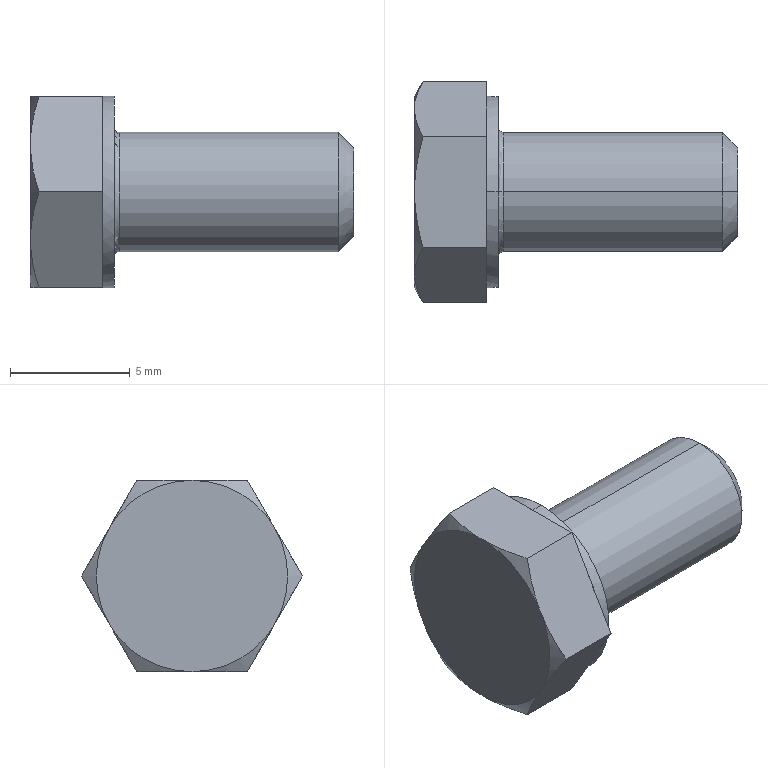Part | SolidWorks | features RevCut 4, Chamfer 1, Extrusion 1, Fillet 1, LPattern 1, Revolution 1 | 1 solid | 29 faces | box 13.5 x 9.238 x 8 mm | volume 384.396 mm3 | plane 15 | cone 8 | cylinder 4 | torus 2 | commonest cylinder face diameters 5 x2 8 x2
STEP:
#1=CARTESIAN_POINT('',(3.7,0.,2.5));
#2=VERTEX_POINT('',#1);
#3=CARTESIAN_POINT('',(3.7,0.,-2.5));
#4=VERTEX_POINT('',#3);
#5=CARTESIAN_POINT('',(3.7,0.,0.));
#6=DIRECTION('',(1.,0.,0.));
#7=DIRECTION('',(0.,0.,-1.));
#8=AXIS2_PLACEMENT_3D('',#5,#6,#7);
#9=CIRCLE('',#8,2.5);
#10=EDGE_CURVE('',#2,#4,#9,.T.);
#11=ORIENTED_EDGE('',*,*,#10,.F.);
#12=CARTESIAN_POINT('',(3.5,0.,2.7));
#13=VERTEX_POINT('',#12);
#14=CARTESIAN_POINT('',(3.7,0.,2.7));
#15=DIRECTION('',(0.,1.,0.));
#16=DIRECTION('',(0.,0.,1.));
#17=AXIS2_PLACEMENT_3D('',#14,#15,#16);
#18=CIRCLE('',#17,0.2);
#19=EDGE_CURVE('',#2,#13,#18,.T.);
#20=ORIENTED_EDGE('',*,*,#19,.T.);
#21=CARTESIAN_POINT('',(3.5,0.,-2.7));
#22=VERTEX_POINT('',#21);
#23=CARTESIAN_POINT('',(3.5,0.,0.));
#24=DIRECTION('',(-1.,0.,0.));
#25=DIRECTION('',(0.,0.,-1.));
#26=AXIS2_PLACEMENT_3D('',#23,#24,#25);
#27=CIRCLE('',#26,2.7);
#28=EDGE_CURVE('',#22,#13,#27,.T.);
#29=ORIENTED_EDGE('',*,*,#28,.F.);
#30=CARTESIAN_POINT('',(3.7,0.,-2.7));
#31=DIRECTION('',(0.,-1.,0.));
#32=DIRECTION('',(0.,0.,-1.));
#33=AXIS2_PLACEMENT_3D('',#30,#31,#32);
#34=CIRCLE('',#33,0.2);
#35=EDGE_CURVE('',#4,#22,#34,.T.);
#36=ORIENTED_EDGE('',*,*,#35,.F.);
#37=EDGE_LOOP('',(#11,#20,#29,#36));
#38=FACE_OUTER_BOUND('',#37,.T.);
#39=CARTESIAN_POINT('',(3.7,0.,0.));
#40=DIRECTION('',(1.,0.,0.));
#41=DIRECTION('',(0.,0.,-1.));
#42=AXIS2_PLACEMENT_3D('',#39,#40,#41);
#43=TOROIDAL_SURFACE('',#42,2.7,0.2);
#44=ADVANCED_FACE('',(#38),#43,.F.);
#45=CARTESIAN_POINT('',(13.5,0.,-1.86));
#46=VERTEX_POINT('',#45);
#47=CARTESIAN_POINT('',(13.5,0.,1.86));
#48=VERTEX_POINT('',#47);
#49=CARTESIAN_POINT('',(13.5,0.,0.));
#50=DIRECTION('',(1.,0.,0.));
#51=DIRECTION('',(0.,0.,1.));
#52=AXIS2_PLACEMENT_3D('',#49,#50,#51);
#53=CIRCLE('',#52,1.86);
#54=EDGE_CURVE('',#46,#48,#53,.T.);
#55=ORIENTED_EDGE('',*,*,#54,.F.);
#56=CARTESIAN_POINT('',(12.86,0.,-2.5));
#57=VERTEX_POINT('',#56);
#58=CARTESIAN_POINT('',(12.86,0.,-2.5));
#59=DIRECTION('',(-0.7071,0.,-0.7071));
#60=VECTOR('',#59,1000.);
#61=LINE('',#58,#60);
#62=EDGE_CURVE('',#46,#57,#61,.T.);
#63=ORIENTED_EDGE('',*,*,#62,.T.);
#64=CARTESIAN_POINT('',(12.86,0.,2.5));
#65=VERTEX_POINT('',#64);
#66=CARTESIAN_POINT('',(12.86,0.,0.));
#67=DIRECTION('',(-1.,0.,0.));
#68=DIRECTION('',(0.,0.,1.));
#69=AXIS2_PLACEMENT_3D('',#66,#67,#68);
#70=CIRCLE('',#69,2.5);
#71=EDGE_CURVE('',#65,#57,#70,.T.);
#72=ORIENTED_EDGE('',*,*,#71,.F.);
#73=CARTESIAN_POINT('',(12.86,0.,2.5));
#74=DIRECTION('',(-0.7071,0.,0.7071));
#75=VECTOR('',#74,1000.);
#76=LINE('',#73,#75);
#77=EDGE_CURVE('',#48,#65,#76,.T.);
#78=ORIENTED_EDGE('',*,*,#77,.F.);
#79=EDGE_LOOP('',(#55,#63,#72,#78));
#80=FACE_OUTER_BOUND('',#79,.T.);
#81=CARTESIAN_POINT('',(12.86,0.,0.));
#82=DIRECTION('',(-1.,0.,0.));
#83=DIRECTION('',(0.,0.,1.));
#84=AXIS2_PLACEMENT_3D('',#81,#82,#83);
#85=CONICAL_SURFACE('',#84,2.5,0.7854);
#86=ADVANCED_FACE('',(#80),#85,.T.);
#87=ORIENTED_EDGE('',*,*,#71,.T.);
#88=CARTESIAN_POINT('',(0.,0.,-2.5));
#89=DIRECTION('',(-1.,0.,0.));
#90=VECTOR('',#89,1000.);
#91=LINE('',#88,#90);
#92=EDGE_CURVE('',#57,#4,#91,.T.);
#93=ORIENTED_EDGE('',*,*,#92,.T.);
#94=CARTESIAN_POINT('',(3.7,0.,0.));
#95=DIRECTION('',(1.,0.,0.));
#96=DIRECTION('',(0.,0.,-1.));
#97=AXIS2_PLACEMENT_3D('',#94,#95,#96);
#98=CIRCLE('',#97,2.5);
#99=EDGE_CURVE('',#4,#2,#98,.T.);
#100=ORIENTED_EDGE('',*,*,#99,.T.);
#101=CARTESIAN_POINT('',(0.,0.,2.5));
#102=DIRECTION('',(-1.,0.,0.));
#103=VECTOR('',#102,1000.);
#104=LINE('',#101,#103);
#105=EDGE_CURVE('',#65,#2,#104,.T.);
#106=ORIENTED_EDGE('',*,*,#105,.F.);
#107=EDGE_LOOP('',(#87,#93,#100,#106));
#108=FACE_OUTER_BOUND('',#107,.T.);
#109=CARTESIAN_POINT('',(0.,0.,0.));
#110=DIRECTION('',(-1.,0.,0.));
#111=DIRECTION('',(0.,0.,1.));
#112=AXIS2_PLACEMENT_3D('',#109,#110,#111);
#113=CYLINDRICAL_SURFACE('',#112,2.5);
#114=ADVANCED_FACE('',(#108),#113,.T.);
#115=CARTESIAN_POINT('',(3.5,0.,-4.));
#116=VERTEX_POINT('',#115);
#117=CARTESIAN_POINT('',(3.5,0.,4.));
#118=VERTEX_POINT('',#117);
#119=CARTESIAN_POINT('',(3.5,0.,0.));
#120=DIRECTION('',(1.,0.,0.));
#121=DIRECTION('',(0.,0.,-1.));
#122=AXIS2_PLACEMENT_3D('',#119,#120,#121);
#123=CIRCLE('',#122,4.);
#124=EDGE_CURVE('',#116,#118,#123,.T.);
#125=ORIENTED_EDGE('',*,*,#124,.F.);
#126=CARTESIAN_POINT('',(3.,0.,-4.));
#127=VERTEX_POINT('',#126);
#128=CARTESIAN_POINT('',(0.,0.,-4.));
#129=DIRECTION('',(-1.,0.,0.));
#130=VECTOR('',#129,1000.);
#131=LINE('',#128,#130);
#132=EDGE_CURVE('',#116,#127,#131,.T.);
#133=ORIENTED_EDGE('',*,*,#132,.T.);
#134=CARTESIAN_POINT('',(3.,3.464,-2.));
#135=VERTEX_POINT('',#134);
#136=CARTESIAN_POINT('',(3.,0.,0.));
#137=DIRECTION('',(-1.,0.,0.));
#138=DIRECTION('',(0.,0.,1.));
#139=AXIS2_PLACEMENT_3D('',#136,#137,#138);
#140=CIRCLE('',#139,4.);
#141=EDGE_CURVE('',#135,#127,#140,.T.);
#142=ORIENTED_EDGE('',*,*,#141,.F.);
#143=CARTESIAN_POINT('',(3.,3.464,2.));
#144=VERTEX_POINT('',#143);
#145=CARTESIAN_POINT('',(3.,0.,0.));
#146=DIRECTION('',(-1.,0.,0.));
#147=DIRECTION('',(0.,0.,1.));
#148=AXIS2_PLACEMENT_3D('',#145,#146,#147);
#149=CIRCLE('',#148,4.);
#150=EDGE_CURVE('',#144,#135,#149,.T.);
#151=ORIENTED_EDGE('',*,*,#150,.F.);
#152=CARTESIAN_POINT('',(3.,0.,4.));
#153=VERTEX_POINT('',#152);
#154=CARTESIAN_POINT('',(3.,0.,0.));
#155=DIRECTION('',(-1.,0.,0.));
#156=DIRECTION('',(0.,0.,1.));
#157=AXIS2_PLACEMENT_3D('',#154,#155,#156);
#158=CIRCLE('',#157,4.);
#159=EDGE_CURVE('',#153,#144,#158,.T.);
#160=ORIENTED_EDGE('',*,*,#159,.F.);
#161=CARTESIAN_POINT('',(0.,0.,4.));
#162=DIRECTION('',(-1.,0.,0.));
#163=VECTOR('',#162,1000.);
#164=LINE('',#161,#163);
#165=EDGE_CURVE('',#118,#153,#164,.T.);
#166=ORIENTED_EDGE('',*,*,#165,.F.);
#167=EDGE_LOOP('',(#125,#133,#142,#151,#160,#166));
#168=FACE_OUTER_BOUND('',#167,.T.);
#169=CARTESIAN_POINT('',(0.,0.,0.));
#170=DIRECTION('',(-1.,0.,0.));
#171=DIRECTION('',(0.,0.,1.));
#172=AXIS2_PLACEMENT_3D('',#169,#170,#171);
#173=CYLINDRICAL_SURFACE('',#172,4.);
#174=ADVANCED_FACE('',(#168),#173,.T.);
#175=CARTESIAN_POINT('',(3.,2.309,-4.));
#176=VERTEX_POINT('',#175);
#177=CARTESIAN_POINT('',(3.,2.309,-4.));
#178=DIRECTION('',(0.,0.5,0.866));
#179=VECTOR('',#178,1000.);
#180=LINE('',#177,#179);
#181=EDGE_CURVE('',#176,#135,#180,.T.);
#182=ORIENTED_EDGE('',*,*,#181,.F.);
#183=CARTESIAN_POINT('',(0.3573,2.309,-4.));
#184=VERTEX_POINT('',#183);
#185=CARTESIAN_POINT('',(3.5,2.309,-4.));
#186=DIRECTION('',(-1.,0.,0.));
#187=VECTOR('',#186,1000.);
#188=LINE('',#185,#187);
#189=EDGE_CURVE('',#176,#184,#188,.T.);
#190=ORIENTED_EDGE('',*,*,#189,.T.);
#191=CARTESIAN_POINT('',(0.,3.464,-2.));
#192=VERTEX_POINT('',#191);
#193=CARTESIAN_POINT('',(0.,3.464,-2.));
#194=CARTESIAN_POINT('',(0.,3.268,-2.339));
#195=CARTESIAN_POINT('',(0.03421,3.072,-2.678));
#196=CARTESIAN_POINT('',(0.1587,2.688,-3.345));
#197=CARTESIAN_POINT('',(0.2485,2.498,-3.674));
#198=CARTESIAN_POINT('',(0.3573,2.309,-4.));
#199=B_SPLINE_CURVE_WITH_KNOTS('',3,(#193,#194,#195,#196,#197,#198),.UNSPECIFIED.,.F.,.F.,(4,2,4),(0.002337,0.003501,0.004665),.UNSPECIFIED.);
#200=EDGE_CURVE('',#192,#184,#199,.T.);
#201=ORIENTED_EDGE('',*,*,#200,.F.);
#202=CARTESIAN_POINT('',(0.3573,4.619,0.));
#203=VERTEX_POINT('',#202);
#204=CARTESIAN_POINT('',(0.3573,4.619,0.));
#205=CARTESIAN_POINT('',(0.1392,4.241,-0.6543));
#206=CARTESIAN_POINT('',(0.,3.858,-1.319));
#207=CARTESIAN_POINT('',(0.,3.464,-2.));
#208=B_SPLINE_CURVE_WITH_KNOTS('',3,(#204,#205,#206,#207),.UNSPECIFIED.,.F.,.F.,(4,4),(0.000000238,0.002337),.UNSPECIFIED.);
#209=EDGE_CURVE('',#203,#192,#208,.T.);
#210=ORIENTED_EDGE('',*,*,#209,.F.);
#211=CARTESIAN_POINT('',(3.,4.619,0.));
#212=VERTEX_POINT('',#211);
#213=CARTESIAN_POINT('',(3.5,4.619,0.));
#214=DIRECTION('',(-1.,0.,0.));
#215=VECTOR('',#214,1000.);
#216=LINE('',#213,#215);
#217=EDGE_CURVE('',#212,#203,#216,.T.);
#218=ORIENTED_EDGE('',*,*,#217,.F.);
#219=CARTESIAN_POINT('',(3.,2.309,-4.));
#220=DIRECTION('',(0.,0.5,0.866));
#221=VECTOR('',#220,1000.);
#222=LINE('',#219,#221);
#223=EDGE_CURVE('',#135,#212,#222,.T.);
#224=ORIENTED_EDGE('',*,*,#223,.F.);
#225=EDGE_LOOP('',(#182,#190,#201,#210,#218,#224));
#226=FACE_OUTER_BOUND('',#225,.T.);
#227=CARTESIAN_POINT('',(3.5,2.309,-4.));
#228=DIRECTION('',(0.,-0.866,0.5));
#229=DIRECTION('',(0.,-0.5,-0.866));
#230=AXIS2_PLACEMENT_3D('',#227,#228,#229);
#231=PLANE('',#230);
#232=ADVANCED_FACE('',(#226),#231,.F.);
#233=CARTESIAN_POINT('',(3.,4.619,0.));
#234=DIRECTION('',(0.,-0.5,0.866));
#235=VECTOR('',#234,1000.);
#236=LINE('',#233,#235);
#237=EDGE_CURVE('',#212,#144,#236,.T.);
#238=ORIENTED_EDGE('',*,*,#237,.F.);
#239=ORIENTED_EDGE('',*,*,#217,.T.);
#240=CARTESIAN_POINT('',(0.,3.464,2.));
#241=VERTEX_POINT('',#240);
#242=CARTESIAN_POINT('',(0.,3.464,2.));
#243=CARTESIAN_POINT('',(0.,3.66,1.661));
#244=CARTESIAN_POINT('',(0.03421,3.856,1.322));
#245=CARTESIAN_POINT('',(0.1587,4.24,0.6554));
#246=CARTESIAN_POINT('',(0.2485,4.43,0.3264));
#247=CARTESIAN_POINT('',(0.3573,4.619,0.));
#248=B_SPLINE_CURVE_WITH_KNOTS('',3,(#242,#243,#244,#245,#246,#247),.UNSPECIFIED.,.F.,.F.,(4,2,4),(0.002337,0.003501,0.004665),.UNSPECIFIED.);
#249=EDGE_CURVE('',#241,#203,#248,.T.);
#250=ORIENTED_EDGE('',*,*,#249,.F.);
#251=CARTESIAN_POINT('',(0.3573,2.309,4.));
#252=VERTEX_POINT('',#251);
#253=CARTESIAN_POINT('',(0.3573,2.309,4.));
#254=CARTESIAN_POINT('',(0.1392,2.687,3.346));
#255=CARTESIAN_POINT('',(0.,3.071,2.681));
#256=CARTESIAN_POINT('',(0.,3.464,2.));
#257=B_SPLINE_CURVE_WITH_KNOTS('',3,(#253,#254,#255,#256),.UNSPECIFIED.,.F.,.F.,(4,4),(0.000000238,0.002337),.UNSPECIFIED.);
#258=EDGE_CURVE('',#252,#241,#257,.T.);
#259=ORIENTED_EDGE('',*,*,#258,.F.);
#260=CARTESIAN_POINT('',(3.,2.309,4.));
#261=VERTEX_POINT('',#260);
#262=CARTESIAN_POINT('',(3.5,2.309,4.));
#263=DIRECTION('',(-1.,0.,0.));
#264=VECTOR('',#263,1000.);
#265=LINE('',#262,#264);
#266=EDGE_CURVE('',#261,#252,#265,.T.);
#267=ORIENTED_EDGE('',*,*,#266,.F.);
#268=CARTESIAN_POINT('',(3.,4.619,0.));
#269=DIRECTION('',(0.,-0.5,0.866));
#270=VECTOR('',#269,1000.);
#271=LINE('',#268,#270);
#272=EDGE_CURVE('',#144,#261,#271,.T.);
#273=ORIENTED_EDGE('',*,*,#272,.F.);
#274=EDGE_LOOP('',(#238,#239,#250,#259,#267,#273));
#275=FACE_OUTER_BOUND('',#274,.T.);
#276=CARTESIAN_POINT('',(3.5,4.619,0.));
#277=DIRECTION('',(0.,-0.866,-0.5));
#278=DIRECTION('',(0.,0.5,-0.866));
#279=AXIS2_PLACEMENT_3D('',#276,#277,#278);
#280=PLANE('',#279);
#281=ADVANCED_FACE('',(#275),#280,.F.);
#282=CARTESIAN_POINT('',(3.,2.309,4.));
#283=DIRECTION('',(0.,-1.,0.));
#284=VECTOR('',#283,1000.);
#285=LINE('',#282,#284);
#286=EDGE_CURVE('',#261,#153,#285,.T.);
#287=ORIENTED_EDGE('',*,*,#286,.F.);
#288=ORIENTED_EDGE('',*,*,#266,.T.);
#289=CARTESIAN_POINT('',(0.,0.,4.));
#290=VERTEX_POINT('',#289);
#291=CARTESIAN_POINT('',(0.,0.,4.));
#292=CARTESIAN_POINT('',(0.,0.3912,4.));
#293=CARTESIAN_POINT('',(0.03459,0.7871,4.));
#294=CARTESIAN_POINT('',(0.1597,1.558,4.));
#295=CARTESIAN_POINT('',(0.2494,1.936,4.));
#296=CARTESIAN_POINT('',(0.3573,2.309,4.));
#297=B_SPLINE_CURVE_WITH_KNOTS('',3,(#291,#292,#293,#294,#295,#296),.UNSPECIFIED.,.F.,.F.,(4,2,4),(0.006655,0.007825,0.008995),.UNSPECIFIED.);
#298=EDGE_CURVE('',#290,#252,#297,.T.);
#299=ORIENTED_EDGE('',*,*,#298,.F.);
#300=CARTESIAN_POINT('',(0.3573,-2.309,4.));
#301=VERTEX_POINT('',#300);
#302=CARTESIAN_POINT('',(0.3573,-2.309,4.));
#303=CARTESIAN_POINT('',(0.2487,-1.933,4.));
#304=CARTESIAN_POINT('',(0.1579,-1.549,4.));
#305=CARTESIAN_POINT('',(0.03364,-0.7786,4.));
#306=CARTESIAN_POINT('',(0.,-0.3909,4.));
#307=CARTESIAN_POINT('',(0.,0.,4.));
#308=B_SPLINE_CURVE_WITH_KNOTS('',3,(#302,#303,#304,#305,#306,#307),.UNSPECIFIED.,.F.,.F.,(4,2,4),(0.004317,0.005486,0.006655),.UNSPECIFIED.);
#309=EDGE_CURVE('',#301,#290,#308,.T.);
#310=ORIENTED_EDGE('',*,*,#309,.F.);
#311=CARTESIAN_POINT('',(3.,-2.309,4.));
#312=VERTEX_POINT('',#311);
#313=CARTESIAN_POINT('',(3.5,-2.309,4.));
#314=DIRECTION('',(-1.,0.,0.));
#315=VECTOR('',#314,1000.);
#316=LINE('',#313,#315);
#317=EDGE_CURVE('',#312,#301,#316,.T.);
#318=ORIENTED_EDGE('',*,*,#317,.F.);
#319=CARTESIAN_POINT('',(3.,2.309,4.));
#320=DIRECTION('',(0.,-1.,0.));
#321=VECTOR('',#320,1000.);
#322=LINE('',#319,#321);
#323=EDGE_CURVE('',#153,#312,#322,.T.);
#324=ORIENTED_EDGE('',*,*,#323,.F.);
#325=EDGE_LOOP('',(#287,#288,#299,#310,#318,#324));
#326=FACE_OUTER_BOUND('',#325,.T.);
#327=CARTESIAN_POINT('',(3.5,2.309,4.));
#328=DIRECTION('',(0.,0.,-1.));
#329=DIRECTION('',(0.,1.,0.));
#330=AXIS2_PLACEMENT_3D('',#327,#328,#329);
#331=PLANE('',#330);
#332=ADVANCED_FACE('',(#326),#331,.F.);
#333=CARTESIAN_POINT('',(3.,-3.464,2.));
#334=VERTEX_POINT('',#333);
#335=CARTESIAN_POINT('',(3.,-4.619,0.));
#336=DIRECTION('',(0.,-0.5,-0.866));
#337=VECTOR('',#336,1000.);
#338=LINE('',#335,#337);
#339=EDGE_CURVE('',#312,#334,#338,.T.);
#340=ORIENTED_EDGE('',*,*,#339,.F.);
#341=ORIENTED_EDGE('',*,*,#317,.T.);
#342=CARTESIAN_POINT('',(0.,-3.464,2.));
#343=VERTEX_POINT('',#342);
#344=CARTESIAN_POINT('',(0.,-3.464,2.));
#345=CARTESIAN_POINT('',(0.,-3.268,2.339));
#346=CARTESIAN_POINT('',(0.03421,-3.072,2.678));
#347=CARTESIAN_POINT('',(0.1587,-2.688,3.345));
#348=CARTESIAN_POINT('',(0.2485,-2.498,3.674));
#349=CARTESIAN_POINT('',(0.3573,-2.309,4.));
#350=B_SPLINE_CURVE_WITH_KNOTS('',3,(#344,#345,#346,#347,#348,#349),.UNSPECIFIED.,.F.,.F.,(4,2,4),(0.002337,0.003501,0.004665),.UNSPECIFIED.);
#351=EDGE_CURVE('',#343,#301,#350,.T.);
#352=ORIENTED_EDGE('',*,*,#351,.F.);
#353=CARTESIAN_POINT('',(0.3573,-4.619,0.));
#354=VERTEX_POINT('',#353);
#355=CARTESIAN_POINT('',(0.3573,-4.619,0.));
#356=CARTESIAN_POINT('',(0.1392,-4.241,0.6543));
#357=CARTESIAN_POINT('',(0.,-3.858,1.319));
#358=CARTESIAN_POINT('',(0.,-3.464,2.));
#359=B_SPLINE_CURVE_WITH_KNOTS('',3,(#355,#356,#357,#358),.UNSPECIFIED.,.F.,.F.,(4,4),(0.000000238,0.002337),.UNSPECIFIED.);
#360=EDGE_CURVE('',#354,#343,#359,.T.);
#361=ORIENTED_EDGE('',*,*,#360,.F.);
#362=CARTESIAN_POINT('',(3.,-4.619,0.));
#363=VERTEX_POINT('',#362);
#364=CARTESIAN_POINT('',(3.5,-4.619,0.));
#365=DIRECTION('',(-1.,0.,0.));
#366=VECTOR('',#365,1000.);
#367=LINE('',#364,#366);
#368=EDGE_CURVE('',#363,#354,#367,.T.);
#369=ORIENTED_EDGE('',*,*,#368,.F.);
#370=CARTESIAN_POINT('',(3.,-4.619,0.));
#371=DIRECTION('',(0.,-0.5,-0.866));
#372=VECTOR('',#371,1000.);
#373=LINE('',#370,#372);
#374=EDGE_CURVE('',#334,#363,#373,.T.);
#375=ORIENTED_EDGE('',*,*,#374,.F.);
#376=EDGE_LOOP('',(#340,#341,#352,#361,#369,#375));
#377=FACE_OUTER_BOUND('',#376,.T.);
#378=CARTESIAN_POINT('',(3.5,-4.619,0.));
#379=DIRECTION('',(0.,0.866,-0.5));
#380=DIRECTION('',(0.,0.5,0.866));
#381=AXIS2_PLACEMENT_3D('',#378,#379,#380);
#382=PLANE('',#381);
#383=ADVANCED_FACE('',(#377),#382,.F.);
#384=CARTESIAN_POINT('',(3.,-3.464,-2.));
#385=VERTEX_POINT('',#384);
#386=CARTESIAN_POINT('',(3.,-2.309,-4.));
#387=DIRECTION('',(0.,0.5,-0.866));
#388=VECTOR('',#387,1000.);
#389=LINE('',#386,#388);
#390=EDGE_CURVE('',#363,#385,#389,.T.);
#391=ORIENTED_EDGE('',*,*,#390,.F.);
#392=ORIENTED_EDGE('',*,*,#368,.T.);
#393=CARTESIAN_POINT('',(0.,-3.464,-2.));
#394=VERTEX_POINT('',#393);
#395=CARTESIAN_POINT('',(0.,-3.464,-2.));
#396=CARTESIAN_POINT('',(0.,-3.66,-1.661));
#397=CARTESIAN_POINT('',(0.03421,-3.856,-1.322));
#398=CARTESIAN_POINT('',(0.1587,-4.24,-0.6554));
#399=CARTESIAN_POINT('',(0.2485,-4.43,-0.3264));
#400=CARTESIAN_POINT('',(0.3573,-4.619,0.));
#401=B_SPLINE_CURVE_WITH_KNOTS('',3,(#395,#396,#397,#398,#399,#400),.UNSPECIFIED.,.F.,.F.,(4,2,4),(0.002337,0.003501,0.004665),.UNSPECIFIED.);
#402=EDGE_CURVE('',#394,#354,#401,.T.);
#403=ORIENTED_EDGE('',*,*,#402,.F.);
#404=CARTESIAN_POINT('',(0.3573,-2.309,-4.));
#405=VERTEX_POINT('',#404);
#406=CARTESIAN_POINT('',(0.3573,-2.309,-4.));
#407=CARTESIAN_POINT('',(0.1392,-2.687,-3.346));
#408=CARTESIAN_POINT('',(0.,-3.071,-2.681));
#409=CARTESIAN_POINT('',(0.,-3.464,-2.));
#410=B_SPLINE_CURVE_WITH_KNOTS('',3,(#406,#407,#408,#409),.UNSPECIFIED.,.F.,.F.,(4,4),(0.000000238,0.002337),.UNSPECIFIED.);
#411=EDGE_CURVE('',#405,#394,#410,.T.);
#412=ORIENTED_EDGE('',*,*,#411,.F.);
#413=CARTESIAN_POINT('',(3.,-2.309,-4.));
#414=VERTEX_POINT('',#413);
#415=CARTESIAN_POINT('',(3.5,-2.309,-4.));
#416=DIRECTION('',(-1.,0.,0.));
#417=VECTOR('',#416,1000.);
#418=LINE('',#415,#417);
#419=EDGE_CURVE('',#414,#405,#418,.T.);
#420=ORIENTED_EDGE('',*,*,#419,.F.);
#421=CARTESIAN_POINT('',(3.,-2.309,-4.));
#422=DIRECTION('',(0.,0.5,-0.866));
#423=VECTOR('',#422,1000.);
#424=LINE('',#421,#423);
#425=EDGE_CURVE('',#385,#414,#424,.T.);
#426=ORIENTED_EDGE('',*,*,#425,.F.);
#427=EDGE_LOOP('',(#391,#392,#403,#412,#420,#426));
#428=FACE_OUTER_BOUND('',#427,.T.);
#429=CARTESIAN_POINT('',(3.5,-2.309,-4.));
#430=DIRECTION('',(0.,0.866,0.5));
#431=DIRECTION('',(0.,-0.5,0.866));
#432=AXIS2_PLACEMENT_3D('',#429,#430,#431);
#433=PLANE('',#432);
#434=ADVANCED_FACE('',(#428),#433,.F.);
#435=CARTESIAN_POINT('',(3.,2.309,-4.));
#436=DIRECTION('',(0.,1.,0.));
#437=VECTOR('',#436,1000.);
#438=LINE('',#435,#437);
#439=EDGE_CURVE('',#414,#127,#438,.T.);
#440=ORIENTED_EDGE('',*,*,#439,.F.);
#441=ORIENTED_EDGE('',*,*,#419,.T.);
#442=CARTESIAN_POINT('',(0.,0.,-4.));
#443=VERTEX_POINT('',#442);
#444=CARTESIAN_POINT('',(0.,0.,-4.));
#445=CARTESIAN_POINT('',(0.,-0.3909,-4.));
#446=CARTESIAN_POINT('',(0.03364,-0.7786,-4.));
#447=CARTESIAN_POINT('',(0.1579,-1.549,-4.));
#448=CARTESIAN_POINT('',(0.2487,-1.933,-4.));
#449=CARTESIAN_POINT('',(0.3573,-2.309,-4.));
#450=B_SPLINE_CURVE_WITH_KNOTS('',3,(#444,#445,#446,#447,#448,#449),.UNSPECIFIED.,.F.,.F.,(4,2,4),(0.01471,0.01588,0.01705),.UNSPECIFIED.);
#451=EDGE_CURVE('',#443,#405,#450,.T.);
#452=ORIENTED_EDGE('',*,*,#451,.F.);
#453=CARTESIAN_POINT('',(0.3573,2.309,-4.));
#454=CARTESIAN_POINT('',(0.2494,1.936,-4.));
#455=CARTESIAN_POINT('',(0.1597,1.558,-4.));
#456=CARTESIAN_POINT('',(0.03459,0.7871,-4.));
#457=CARTESIAN_POINT('',(0.,0.3912,-4.));
#458=CARTESIAN_POINT('',(0.,0.,-4.));
#459=B_SPLINE_CURVE_WITH_KNOTS('',3,(#453,#454,#455,#456,#457,#458),.UNSPECIFIED.,.F.,.F.,(4,2,4),(0.01237,0.01354,0.01471),.UNSPECIFIED.);
#460=EDGE_CURVE('',#184,#443,#459,.T.);
#461=ORIENTED_EDGE('',*,*,#460,.F.);
#462=ORIENTED_EDGE('',*,*,#189,.F.);
#463=CARTESIAN_POINT('',(3.,2.309,-4.));
#464=DIRECTION('',(0.,1.,0.));
#465=VECTOR('',#464,1000.);
#466=LINE('',#463,#465);
#467=EDGE_CURVE('',#127,#176,#466,.T.);
#468=ORIENTED_EDGE('',*,*,#467,.F.);
#469=EDGE_LOOP('',(#440,#441,#452,#461,#462,#468));
#470=FACE_OUTER_BOUND('',#469,.T.);
#471=CARTESIAN_POINT('',(3.5,2.309,-4.));
#472=DIRECTION('',(0.,0.,1.));
#473=DIRECTION('',(0.,-1.,0.));
#474=AXIS2_PLACEMENT_3D('',#471,#472,#473);
#475=PLANE('',#474);
#476=ADVANCED_FACE('',(#470),#475,.F.);
#477=ORIENTED_EDGE('',*,*,#411,.T.);
#478=CARTESIAN_POINT('',(0.,0.,0.));
#479=DIRECTION('',(1.,0.,0.));
#480=DIRECTION('',(0.,0.,-1.));
#481=AXIS2_PLACEMENT_3D('',#478,#479,#480);
#482=CIRCLE('',#481,4.);
#483=EDGE_CURVE('',#394,#443,#482,.T.);
#484=ORIENTED_EDGE('',*,*,#483,.T.);
#485=ORIENTED_EDGE('',*,*,#451,.T.);
#486=EDGE_LOOP('',(#477,#484,#485));
#487=FACE_OUTER_BOUND('',#486,.T.);
#488=CARTESIAN_POINT('',(0.,0.,0.));
#489=DIRECTION('',(1.,0.,0.));
#490=DIRECTION('',(0.,0.,-1.));
#491=AXIS2_PLACEMENT_3D('',#488,#489,#490);
#492=CONICAL_SURFACE('',#491,4.,1.047);
#493=ADVANCED_FACE('',(#487),#492,.T.);
#494=ORIENTED_EDGE('',*,*,#360,.T.);
#495=CARTESIAN_POINT('',(0.,0.,0.));
#496=DIRECTION('',(1.,0.,0.));
#497=DIRECTION('',(0.,0.,-1.));
#498=AXIS2_PLACEMENT_3D('',#495,#496,#497);
#499=CIRCLE('',#498,4.);
#500=EDGE_CURVE('',#343,#394,#499,.T.);
#501=ORIENTED_EDGE('',*,*,#500,.T.);
#502=ORIENTED_EDGE('',*,*,#402,.T.);
#503=EDGE_LOOP('',(#494,#501,#502));
#504=FACE_OUTER_BOUND('',#503,.T.);
#505=CARTESIAN_POINT('',(0.,0.,0.));
#506=DIRECTION('',(1.,0.,0.));
#507=DIRECTION('',(0.,0.,-1.));
#508=AXIS2_PLACEMENT_3D('',#505,#506,#507);
#509=CONICAL_SURFACE('',#508,4.,1.047);
#510=ADVANCED_FACE('',(#504),#509,.T.);
#511=ORIENTED_EDGE('',*,*,#309,.T.);
#512=CARTESIAN_POINT('',(0.,0.,0.));
#513=DIRECTION('',(1.,0.,0.));
#514=DIRECTION('',(0.,0.,-1.));
#515=AXIS2_PLACEMENT_3D('',#512,#513,#514);
#516=CIRCLE('',#515,4.);
#517=EDGE_CURVE('',#290,#343,#516,.T.);
#518=ORIENTED_EDGE('',*,*,#517,.T.);
#519=ORIENTED_EDGE('',*,*,#351,.T.);
#520=EDGE_LOOP('',(#511,#518,#519));
#521=FACE_OUTER_BOUND('',#520,.T.);
#522=CARTESIAN_POINT('',(0.,0.,0.));
#523=DIRECTION('',(1.,0.,0.));
#524=DIRECTION('',(0.,0.,-1.));
#525=AXIS2_PLACEMENT_3D('',#522,#523,#524);
#526=CONICAL_SURFACE('',#525,4.,1.047);
#527=ADVANCED_FACE('',(#521),#526,.T.);
#528=ORIENTED_EDGE('',*,*,#298,.T.);
#529=ORIENTED_EDGE('',*,*,#258,.T.);
#530=CARTESIAN_POINT('',(0.,0.,0.));
#531=DIRECTION('',(-1.,0.,0.));
#532=DIRECTION('',(0.,0.,1.));
#533=AXIS2_PLACEMENT_3D('',#530,#531,#532);
#534=CIRCLE('',#533,4.);
#535=EDGE_CURVE('',#290,#241,#534,.T.);
#536=ORIENTED_EDGE('',*,*,#535,.F.);
#537=EDGE_LOOP('',(#528,#529,#536));
#538=FACE_OUTER_BOUND('',#537,.T.);
#539=CARTESIAN_POINT('',(0.,0.,0.));
#540=DIRECTION('',(1.,0.,0.));
#541=DIRECTION('',(0.,0.,-1.));
#542=AXIS2_PLACEMENT_3D('',#539,#540,#541);
#543=CONICAL_SURFACE('',#542,4.,1.047);
#544=ADVANCED_FACE('',(#538),#543,.T.);
#545=ORIENTED_EDGE('',*,*,#249,.T.);
#546=ORIENTED_EDGE('',*,*,#209,.T.);
#547=CARTESIAN_POINT('',(0.,0.,0.));
#548=DIRECTION('',(1.,0.,0.));
#549=DIRECTION('',(0.,0.,-1.));
#550=AXIS2_PLACEMENT_3D('',#547,#548,#549);
#551=CIRCLE('',#550,4.);
#552=EDGE_CURVE('',#192,#241,#551,.T.);
#553=ORIENTED_EDGE('',*,*,#552,.T.);
#554=EDGE_LOOP('',(#545,#546,#553));
#555=FACE_OUTER_BOUND('',#554,.T.);
#556=CARTESIAN_POINT('',(0.,0.,0.));
#557=DIRECTION('',(1.,0.,0.));
#558=DIRECTION('',(0.,0.,-1.));
#559=AXIS2_PLACEMENT_3D('',#556,#557,#558);
#560=CONICAL_SURFACE('',#559,4.,1.047);
#561=ADVANCED_FACE('',(#555),#560,.T.);
#562=ORIENTED_EDGE('',*,*,#200,.T.);
#563=ORIENTED_EDGE('',*,*,#460,.T.);
#564=CARTESIAN_POINT('',(0.,0.,0.));
#565=DIRECTION('',(1.,0.,0.));
#566=DIRECTION('',(0.,0.,-1.));
#567=AXIS2_PLACEMENT_3D('',#564,#565,#566);
#568=CIRCLE('',#567,4.);
#569=EDGE_CURVE('',#443,#192,#568,.T.);
#570=ORIENTED_EDGE('',*,*,#569,.T.);
#571=EDGE_LOOP('',(#562,#563,#570));
#572=FACE_OUTER_BOUND('',#571,.T.);
#573=CARTESIAN_POINT('',(0.,0.,0.));
#574=DIRECTION('',(1.,0.,0.));
#575=DIRECTION('',(0.,0.,-1.));
#576=AXIS2_PLACEMENT_3D('',#573,#574,#575);
#577=CONICAL_SURFACE('',#576,4.,1.047);
#578=ADVANCED_FACE('',(#572),#577,.T.);
#579=ORIENTED_EDGE('',*,*,#569,.F.);
#580=ORIENTED_EDGE('',*,*,#483,.F.);
#581=ORIENTED_EDGE('',*,*,#500,.F.);
#582=ORIENTED_EDGE('',*,*,#517,.F.);
#583=ORIENTED_EDGE('',*,*,#535,.T.);
#584=ORIENTED_EDGE('',*,*,#552,.F.);
#585=EDGE_LOOP('',(#579,#580,#581,#582,#583,#584));
#586=FACE_OUTER_BOUND('',#585,.T.);
#587=CARTESIAN_POINT('',(0.,4.619,0.));
#588=DIRECTION('',(1.,0.,0.));
#589=DIRECTION('',(0.,0.,-1.));
#590=AXIS2_PLACEMENT_3D('',#587,#588,#589);
#591=PLANE('',#590);
#592=ADVANCED_FACE('',(#586),#591,.F.);
#593=ORIENTED_EDGE('',*,*,#181,.T.);
#594=ORIENTED_EDGE('',*,*,#141,.T.);
#595=ORIENTED_EDGE('',*,*,#467,.T.);
#596=EDGE_LOOP('',(#593,#594,#595));
#597=FACE_OUTER_BOUND('',#596,.T.);
#598=CARTESIAN_POINT('',(3.,4.,0.));
#599=DIRECTION('',(1.,0.,0.));
#600=DIRECTION('',(0.,0.,-1.));
#601=AXIS2_PLACEMENT_3D('',#598,#599,#600);
#602=PLANE('',#601);
#603=ADVANCED_FACE('',(#597),#602,.T.);
#604=ORIENTED_EDGE('',*,*,#223,.T.);
#605=ORIENTED_EDGE('',*,*,#237,.T.);
#606=ORIENTED_EDGE('',*,*,#150,.T.);
#607=EDGE_LOOP('',(#604,#605,#606));
#608=FACE_OUTER_BOUND('',#607,.T.);
#609=CARTESIAN_POINT('',(3.,4.,0.));
#610=DIRECTION('',(1.,0.,0.));
#611=DIRECTION('',(0.,0.,-1.));
#612=AXIS2_PLACEMENT_3D('',#609,#610,#611);
#613=PLANE('',#612);
#614=ADVANCED_FACE('',(#608),#613,.T.);
#615=ORIENTED_EDGE('',*,*,#272,.T.);
#616=ORIENTED_EDGE('',*,*,#286,.T.);
#617=ORIENTED_EDGE('',*,*,#159,.T.);
#618=EDGE_LOOP('',(#615,#616,#617));
#619=FACE_OUTER_BOUND('',#618,.T.);
#620=CARTESIAN_POINT('',(3.,4.,0.));
#621=DIRECTION('',(1.,0.,0.));
#622=DIRECTION('',(0.,0.,-1.));
#623=AXIS2_PLACEMENT_3D('',#620,#621,#622);
#624=PLANE('',#623);
#625=ADVANCED_FACE('',(#619),#624,.T.);
#626=ORIENTED_EDGE('',*,*,#323,.T.);
#627=ORIENTED_EDGE('',*,*,#339,.T.);
#628=CARTESIAN_POINT('',(3.,0.,0.));
#629=DIRECTION('',(-1.,0.,0.));
#630=DIRECTION('',(0.,0.,1.));
#631=AXIS2_PLACEMENT_3D('',#628,#629,#630);
#632=CIRCLE('',#631,4.);
#633=EDGE_CURVE('',#334,#153,#632,.T.);
#634=ORIENTED_EDGE('',*,*,#633,.T.);
#635=EDGE_LOOP('',(#626,#627,#634));
#636=FACE_OUTER_BOUND('',#635,.T.);
#637=CARTESIAN_POINT('',(3.,4.,0.));
#638=DIRECTION('',(1.,0.,0.));
#639=DIRECTION('',(0.,0.,-1.));
#640=AXIS2_PLACEMENT_3D('',#637,#638,#639);
#641=PLANE('',#640);
#642=ADVANCED_FACE('',(#636),#641,.T.);
#643=ORIENTED_EDGE('',*,*,#374,.T.);
#644=ORIENTED_EDGE('',*,*,#390,.T.);
#645=CARTESIAN_POINT('',(3.,0.,0.));
#646=DIRECTION('',(-1.,0.,0.));
#647=DIRECTION('',(0.,0.,1.));
#648=AXIS2_PLACEMENT_3D('',#645,#646,#647);
#649=CIRCLE('',#648,4.);
#650=EDGE_CURVE('',#385,#334,#649,.T.);
#651=ORIENTED_EDGE('',*,*,#650,.T.);
#652=EDGE_LOOP('',(#643,#644,#651));
#653=FACE_OUTER_BOUND('',#652,.T.);
#654=CARTESIAN_POINT('',(3.,4.,0.));
#655=DIRECTION('',(1.,0.,0.));
#656=DIRECTION('',(0.,0.,-1.));
#657=AXIS2_PLACEMENT_3D('',#654,#655,#656);
#658=PLANE('',#657);
#659=ADVANCED_FACE('',(#653),#658,.T.);
#660=ORIENTED_EDGE('',*,*,#425,.T.);
#661=ORIENTED_EDGE('',*,*,#439,.T.);
#662=CARTESIAN_POINT('',(3.,0.,0.));
#663=DIRECTION('',(-1.,0.,0.));
#664=DIRECTION('',(0.,0.,1.));
#665=AXIS2_PLACEMENT_3D('',#662,#663,#664);
#666=CIRCLE('',#665,4.);
#667=EDGE_CURVE('',#127,#385,#666,.T.);
#668=ORIENTED_EDGE('',*,*,#667,.T.);
#669=EDGE_LOOP('',(#660,#661,#668));
#670=FACE_OUTER_BOUND('',#669,.T.);
#671=CARTESIAN_POINT('',(3.,4.,0.));
#672=DIRECTION('',(1.,0.,0.));
#673=DIRECTION('',(0.,0.,-1.));
#674=AXIS2_PLACEMENT_3D('',#671,#672,#673);
#675=PLANE('',#674);
#676=ADVANCED_FACE('',(#670),#675,.T.);
#677=ORIENTED_EDGE('',*,*,#132,.F.);
#678=CARTESIAN_POINT('',(3.5,0.,0.));
#679=DIRECTION('',(1.,0.,0.));
#680=DIRECTION('',(0.,0.,-1.));
#681=AXIS2_PLACEMENT_3D('',#678,#679,#680);
#682=CIRCLE('',#681,4.);
#683=EDGE_CURVE('',#118,#116,#682,.T.);
#684=ORIENTED_EDGE('',*,*,#683,.F.);
#685=ORIENTED_EDGE('',*,*,#165,.T.);
#686=ORIENTED_EDGE('',*,*,#633,.F.);
#687=ORIENTED_EDGE('',*,*,#650,.F.);
#688=ORIENTED_EDGE('',*,*,#667,.F.);
#689=EDGE_LOOP('',(#677,#684,#685,#686,#687,#688));
#690=FACE_OUTER_BOUND('',#689,.T.);
#691=CARTESIAN_POINT('',(0.,0.,0.));
#692=DIRECTION('',(-1.,0.,0.));
#693=DIRECTION('',(0.,0.,1.));
#694=AXIS2_PLACEMENT_3D('',#691,#692,#693);
#695=CYLINDRICAL_SURFACE('',#694,4.);
#696=ADVANCED_FACE('',(#690),#695,.T.);
#697=CARTESIAN_POINT('',(13.5,0.,0.));
#698=DIRECTION('',(1.,0.,0.));
#699=DIRECTION('',(0.,0.,1.));
#700=AXIS2_PLACEMENT_3D('',#697,#698,#699);
#701=CIRCLE('',#700,1.86);
#702=EDGE_CURVE('',#48,#46,#701,.T.);
#703=ORIENTED_EDGE('',*,*,#702,.T.);
#704=ORIENTED_EDGE('',*,*,#54,.T.);
#705=EDGE_LOOP('',(#703,#704));
#706=FACE_OUTER_BOUND('',#705,.T.);
#707=CARTESIAN_POINT('',(13.5,0.,0.));
#708=DIRECTION('',(-1.,0.,0.));
#709=DIRECTION('',(0.,0.,1.));
#710=AXIS2_PLACEMENT_3D('',#707,#708,#709);
#711=PLANE('',#710);
#712=ADVANCED_FACE('',(#706),#711,.F.);
#713=ORIENTED_EDGE('',*,*,#92,.F.);
#714=CARTESIAN_POINT('',(12.86,0.,0.));
#715=DIRECTION('',(-1.,0.,0.));
#716=DIRECTION('',(0.,0.,1.));
#717=AXIS2_PLACEMENT_3D('',#714,#715,#716);
#718=CIRCLE('',#717,2.5);
#719=EDGE_CURVE('',#57,#65,#718,.T.);
#720=ORIENTED_EDGE('',*,*,#719,.T.);
#721=ORIENTED_EDGE('',*,*,#105,.T.);
#722=ORIENTED_EDGE('',*,*,#10,.T.);
#723=EDGE_LOOP('',(#713,#720,#721,#722));
#724=FACE_OUTER_BOUND('',#723,.T.);
#725=CARTESIAN_POINT('',(0.,0.,0.));
#726=DIRECTION('',(-1.,0.,0.));
#727=DIRECTION('',(0.,0.,1.));
#728=AXIS2_PLACEMENT_3D('',#725,#726,#727);
#729=CYLINDRICAL_SURFACE('',#728,2.5);
#730=ADVANCED_FACE('',(#724),#729,.T.);
#731=ORIENTED_EDGE('',*,*,#28,.T.);
#732=CARTESIAN_POINT('',(3.5,0.,0.));
#733=DIRECTION('',(-1.,0.,0.));
#734=DIRECTION('',(0.,0.,-1.));
#735=AXIS2_PLACEMENT_3D('',#732,#733,#734);
#736=CIRCLE('',#735,2.7);
#737=EDGE_CURVE('',#13,#22,#736,.T.);
#738=ORIENTED_EDGE('',*,*,#737,.T.);
#739=EDGE_LOOP('',(#731,#738));
#740=FACE_BOUND('',#739,.T.);
#741=ORIENTED_EDGE('',*,*,#683,.T.);
#742=ORIENTED_EDGE('',*,*,#124,.T.);
#743=EDGE_LOOP('',(#741,#742));
#744=FACE_OUTER_BOUND('',#743,.T.);
#745=CARTESIAN_POINT('',(3.5,4.619,0.));
#746=DIRECTION('',(1.,0.,0.));
#747=DIRECTION('',(0.,0.,-1.));
#748=AXIS2_PLACEMENT_3D('',#745,#746,#747);
#749=PLANE('',#748);
#750=ADVANCED_FACE('',(#740,#744),#749,.T.);
#751=ORIENTED_EDGE('',*,*,#62,.F.);
#752=ORIENTED_EDGE('',*,*,#702,.F.);
#753=ORIENTED_EDGE('',*,*,#77,.T.);
#754=ORIENTED_EDGE('',*,*,#719,.F.);
#755=EDGE_LOOP('',(#751,#752,#753,#754));
#756=FACE_OUTER_BOUND('',#755,.T.);
#757=CARTESIAN_POINT('',(12.86,0.,0.));
#758=DIRECTION('',(-1.,0.,0.));
#759=DIRECTION('',(0.,0.,1.));
#760=AXIS2_PLACEMENT_3D('',#757,#758,#759);
#761=CONICAL_SURFACE('',#760,2.5,0.7854);
#762=ADVANCED_FACE('',(#756),#761,.T.);
#763=ORIENTED_EDGE('',*,*,#19,.F.);
#764=ORIENTED_EDGE('',*,*,#99,.F.);
#765=ORIENTED_EDGE('',*,*,#35,.T.);
#766=ORIENTED_EDGE('',*,*,#737,.F.);
#767=EDGE_LOOP('',(#763,#764,#765,#766));
#768=FACE_OUTER_BOUND('',#767,.T.);
#769=CARTESIAN_POINT('',(3.7,0.,0.));
#770=DIRECTION('',(1.,0.,0.));
#771=DIRECTION('',(0.,0.,-1.));
#772=AXIS2_PLACEMENT_3D('',#769,#770,#771);
#773=TOROIDAL_SURFACE('',#772,2.7,0.2);
#774=ADVANCED_FACE('',(#768),#773,.F.);
#775=CLOSED_SHELL('',(#44,#86,#114,#174,#232,#281,#332,#383,#434,#476,#493,#510,#527,#544,#561,#578,#592,#603,#614,#625,#642,#659,#676,#696,#712,#730,#750,#762,#774));
#776=MANIFOLD_SOLID_BREP('',#775);
#777=CARTESIAN_POINT('',(0.,0.,0.));
#778=DIRECTION('',(0.,0.,1.));
#779=DIRECTION('',(1.,0.,0.));
#780=AXIS2_PLACEMENT_3D('',#777,#778,#779);
#781=(LENGTH_UNIT()NAMED_UNIT(*)SI_UNIT(.MILLI.,.METRE.));
#782=UNCERTAINTY_MEASURE_WITH_UNIT(LENGTH_MEASURE(0.00001),#781,'','');
#783=(NAMED_UNIT(*)PLANE_ANGLE_UNIT()SI_UNIT($,.RADIAN.));
#784=(NAMED_UNIT(*)SI_UNIT($,.STERADIAN.)SOLID_ANGLE_UNIT());
#785=(GEOMETRIC_REPRESENTATION_CONTEXT(3)GLOBAL_UNCERTAINTY_ASSIGNED_CONTEXT((#782))GLOBAL_UNIT_ASSIGNED_CONTEXT((#781,#783,#784))REPRESENTATION_CONTEXT('',''));
#786=ADVANCED_BREP_SHAPE_REPRESENTATION('',(#776,#780),#785);